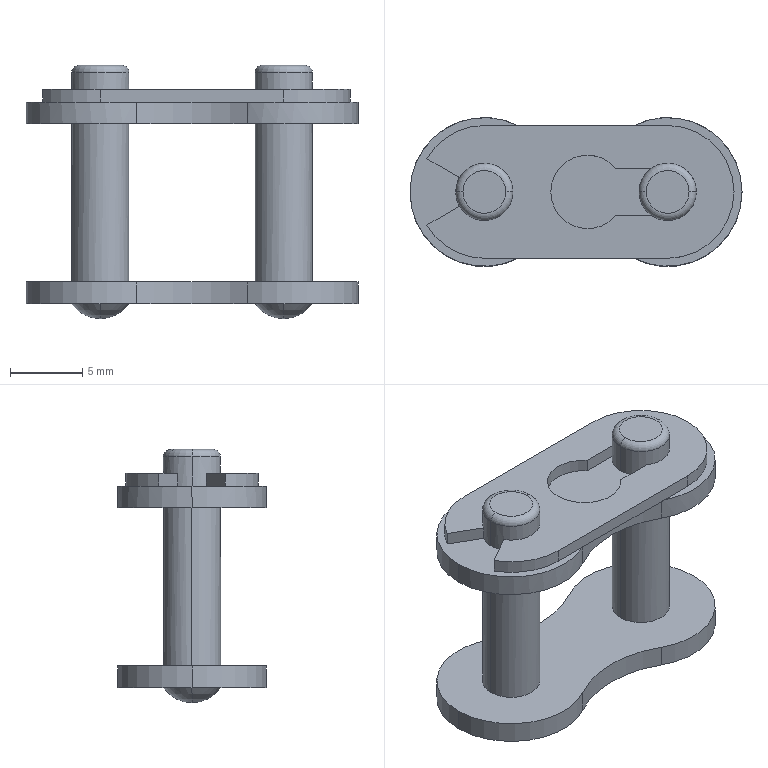Part | STEP file | _JNTC40 | 1 solid | 55 faces | box 23 x 10.3 x 17.55 mm | volume 1033 mm3 | cylinder 26 | plane 17 | sphere 8 | torus 4 | commonest cylinder face diameters 3.97 x8 10.3 x8 9.2 x4 15.788 x4 5.1 x2